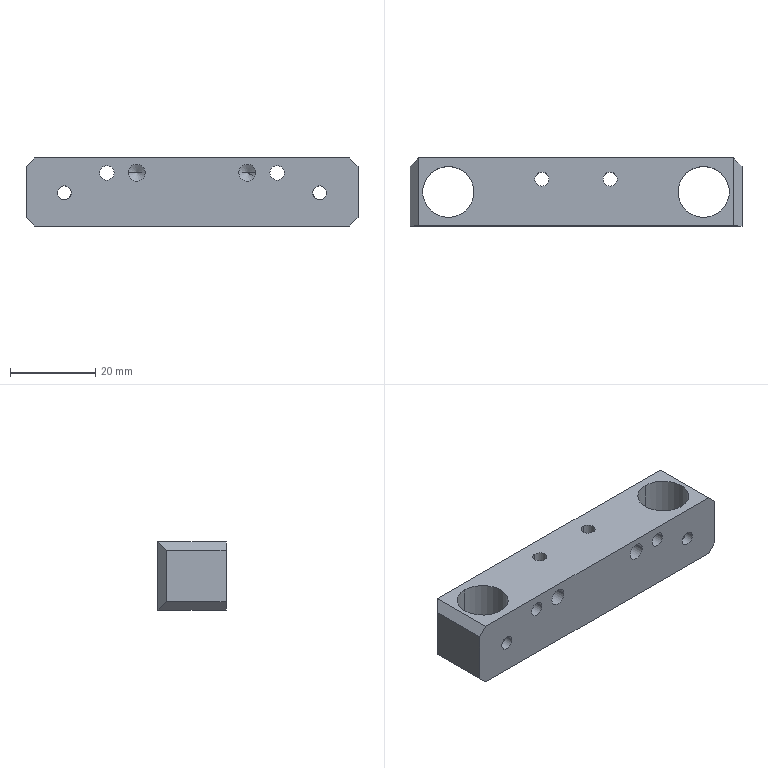NC program | NX | posted with a generic post | part box 78 x 16 x 16 mm
Whole program:
N10 G17 G21 G94 G90
(HOLE_MILLING , TOOL : D4)
N12 T17 M6
N14 G54
N16 G17 G0 G90 X-20. Y-4.5 B0. C0. S5000 M3
N18 G43 Z30. H17
N20 Z0.5
N22 G94 G3 X-19.5 Y-5. R0.5 F1250.
N24 X-19. Y-4.5 R0.5
N26 X-19. Y-4.5 Z0.42 I-1. J0.
N28 X-19. Y-4.5 Z0.34 I-1. J0.
N30 X-19. Y-4.5 Z0.26 I-1. J0.
N32 X-19. Y-4.5 Z0.18 I-1. J0.
N34 X-19. Y-4.5 Z0.1 I-1. J0.
N36 X-19. Y-4.5 Z0.02 I-1. J0.
N38 X-19. Y-4.5 Z-0.06 I-1. J0.
N40 X-19. Y-4.5 Z-0.14 I-1. J0.
N42 X-19. Y-4.5 Z-0.22 I-1. J0.
N44 X-19. Y-4.5 Z-0.3 I-1. J0.
N46 X-19. Y-4.5 Z-0.38 I-1. J0.
N48 X-19. Y-4.5 Z-0.46 I-1. J0.
N50 X-19. Y-4.5 Z-0.54 I-1. J0.
N52 X-19. Y-4.5 Z-0.62 I-1. J0.
N54 X-19. Y-4.5 Z-0.7 I-1. J0.
N56 X-19. Y-4.5 Z-0.78 I-1. J0.
N58 X-19. Y-4.5 Z-0.86 I-1. J0.
N60 X-19. Y-4.5 Z-0.94 I-1. J0.
N62 X-19. Y-4.5 Z-1.02 I-1. J0.
N64 X-19. Y-4.5 Z-1.1 I-1. J0.
N66 X-19. Y-4.5 Z-1.18 I-1. J0.
N68 X-19. Y-4.5 Z-1.26 I-1. J0.
N70 X-19. Y-4.5 Z-1.34 I-1. J0.
N72 X-19. Y-4.5 Z-1.42 I-1. J0.
N74 X-19. Y-4.5 Z-1.5 I-1. J0.
N76 X-19. Y-4.5 Z-1.58 I-1. J0.
N78 X-19. Y-4.5 Z-1.66 I-1. J0.
N80 X-19. Y-4.5 Z-1.74 I-1. J0.
N82 X-19. Y-4.5 Z-1.82 I-1. J0.
N84 X-19. Y-4.5 Z-1.9 I-1. J0.
N86 X-19. Y-4.5 Z-1.98 I-1. J0.
N88 X-19. Y-4.5 Z-2.06 I-1. J0.
N90 X-19. Y-4.5 Z-2.14 I-1. J0.
N92 X-19. Y-4.5 Z-2.22 I-1. J0.
N94 X-19. Y-4.5 Z-2.3 I-1. J0.
N96 X-19. Y-4.5 Z-2.38 I-1. J0.
N98 X-19. Y-4.5 Z-2.46 I-1. J0.
N100 X-19. Y-4.5 Z-2.54 I-1. J0.
N102 X-19. Y-4.5 Z-2.62 I-1. J0.
N104 X-19. Y-4.5 Z-2.7 I-1. J0.
N106 X-19. Y-4.5 Z-2.78 I-1. J0.
N108 X-19. Y-4.5 Z-2.86 I-1. J0.
N110 X-19. Y-4.5 Z-2.94 I-1. J0.
N112 X-19. Y-4.5 Z-3.02 I-1. J0.
N114 X-19. Y-4.5 Z-3.1 I-1. J0.
N116 X-19. Y-4.5 Z-3.18 I-1. J0.
N118 X-19. Y-4.5 Z-3.26 I-1. J0.
N120 X-19. Y-4.5 Z-3.34 I-1. J0.
N122 X-20. Y-5.5 Z-3.4 R-1.
N124 X-19. Y-4.5 R1.
N126 X-20. Y-5.5 R-1.
N128 X-19.5 Y-5. R0.5
N130 X-20. Y-4.5 R0.5
N132 G0 Z30.
N134 X20.
N136 Z0.5
N138 G3 X20.5 Y-5. R0.5
N140 X21. Y-4.5 R0.5
N142 X21. Y-4.5 Z0.42 I-1. J0.
N144 X21. Y-4.5 Z0.34 I-1. J0.
N146 X21. Y-4.5 Z0.26 I-1. J0.
N148 X21. Y-4.5 Z0.18 I-1. J0.
N150 X21. Y-4.5 Z0.1 I-1. J0.
N152 X21. Y-4.5 Z0.02 I-1. J0.
N154 X21. Y-4.5 Z-0.06 I-1. J0.
N156 X21. Y-4.5 Z-0.14 I-1. J0.
N158 X21. Y-4.5 Z-0.22 I-1. J0.
N160 X21. Y-4.5 Z-0.3 I-1. J0.
N162 X21. Y-4.5 Z-0.38 I-1. J0.
N164 X21. Y-4.5 Z-0.46 I-1. J0.
N166 X21. Y-4.5 Z-0.54 I-1. J0.
N168 X21. Y-4.5 Z-0.62 I-1. J0.
N170 X21. Y-4.5 Z-0.7 I-1. J0.
N172 X21. Y-4.5 Z-0.78 I-1. J0.
N174 X21. Y-4.5 Z-0.86 I-1. J0.
N176 X21. Y-4.5 Z-0.94 I-1. J0.
N178 X21. Y-4.5 Z-1.02 I-1. J0.
N180 X21. Y-4.5 Z-1.1 I-1. J0.
N182 X21. Y-4.5 Z-1.18 I-1. J0.
N184 X21. Y-4.5 Z-1.26 I-1. J0.
N186 X21. Y-4.5 Z-1.34 I-1. J0.
N188 X21. Y-4.5 Z-1.42 I-1. J0.
N190 X21. Y-4.5 Z-1.5 I-1. J0.
N192 X21. Y-4.5 Z-1.58 I-1. J0.
N194 X21. Y-4.5 Z-1.66 I-1. J0.
N196 X21. Y-4.5 Z-1.74 I-1. J0.
N198 X21. Y-4.5 Z-1.82 I-1. J0.
N200 X21. Y-4.5 Z-1.9 I-1. J0.
N202 X21. Y-4.5 Z-1.98 I-1. J0.
N204 X21. Y-4.5 Z-2.06 I-1. J0.
N206 X21. Y-4.5 Z-2.14 I-1. J0.
N208 X21. Y-4.5 Z-2.22 I-1. J0.
N210 X21. Y-4.5 Z-2.3 I-1. J0.
N212 X21. Y-4.5 Z-2.38 I-1. J0.
N214 X21. Y-4.5 Z-2.46 I-1. J0.
N216 X21. Y-4.5 Z-2.54 I-1. J0.
N218 X21. Y-4.5 Z-2.62 I-1. J0.
N220 X21. Y-4.5 Z-2.7 I-1. J0.
N222 X21. Y-4.5 Z-2.78 I-1. J0.
N224 X21. Y-4.5 Z-2.86 I-1. J0.
N226 X21. Y-4.5 Z-2.94 I-1. J0.
N228 X21. Y-4.5 Z-3.02 I-1. J0.
N230 X21. Y-4.5 Z-3.1 I-1. J0.
N232 X21. Y-4.5 Z-3.18 I-1. J0.
N234 X21. Y-4.5 Z-3.26 I-1. J0.
N236 X21. Y-4.5 Z-3.34 I-1. J0.
N238 X20. Y-5.5 Z-3.4 R-1.
N240 X21. Y-4.5 R1.
N242 X20. Y-5.5 R-1.
N244 X20.5 Y-5. R0.5
N246 X20. Y-4.5 R0.5
N248 G0 Z30.
N250 M5
N252 M2